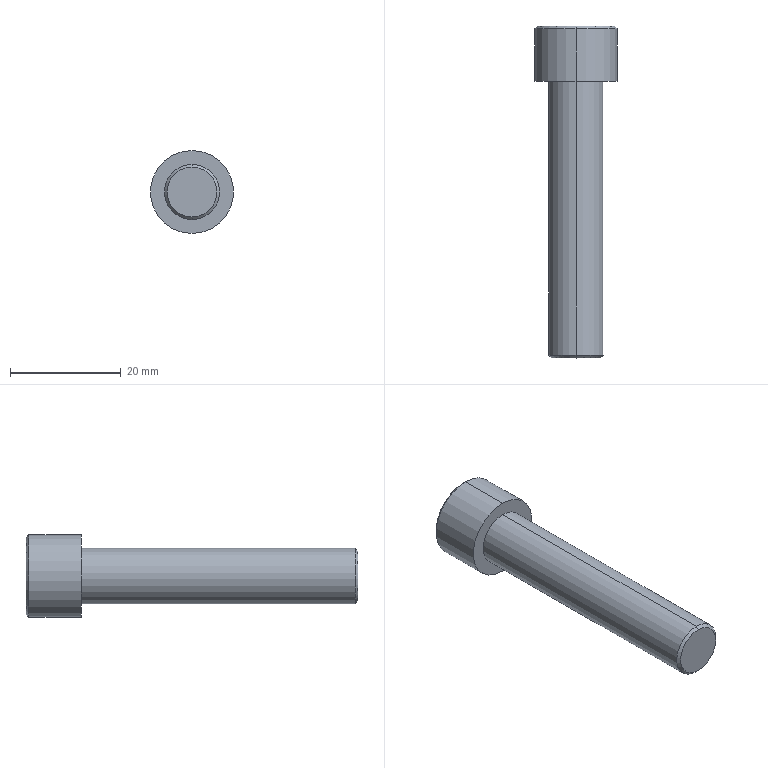Part | SolidWorks | features Chamfer 1, Extrusion 1, ICE 1 | 1 solid | 11 faces | box 15 x 60 x 15 mm | volume 5685 mm3 | cone 4 | cylinder 4 | plane 3 | commonest cylinder face diameters 10 x2 15 x2
STEP:
#1=CARTESIAN_POINT('',(0.,-25.,-4.5));
#2=VERTEX_POINT('',#1);
#3=CARTESIAN_POINT('',(0.,-25.,4.5));
#4=VERTEX_POINT('',#3);
#5=CARTESIAN_POINT('',(0.,-25.,0.));
#6=DIRECTION('',(0.,-1.,0.));
#7=DIRECTION('',(0.,0.,1.));
#8=AXIS2_PLACEMENT_3D('',#5,#6,#7);
#9=CIRCLE('',#8,4.5);
#10=EDGE_CURVE('',#2,#4,#9,.T.);
#11=ORIENTED_EDGE('',*,*,#10,.F.);
#12=CARTESIAN_POINT('',(0.,-24.5,-5.));
#13=VERTEX_POINT('',#12);
#14=CARTESIAN_POINT('',(0.,-24.5,-5.));
#15=DIRECTION('',(0.,0.7071,-0.7071));
#16=VECTOR('',#15,1000.);
#17=LINE('',#14,#16);
#18=EDGE_CURVE('',#2,#13,#17,.T.);
#19=ORIENTED_EDGE('',*,*,#18,.T.);
#20=CARTESIAN_POINT('',(0.,-24.5,5.));
#21=VERTEX_POINT('',#20);
#22=CARTESIAN_POINT('',(0.,-24.5,0.));
#23=DIRECTION('',(0.,1.,0.));
#24=DIRECTION('',(0.,0.,1.));
#25=AXIS2_PLACEMENT_3D('',#22,#23,#24);
#26=CIRCLE('',#25,5.);
#27=EDGE_CURVE('',#21,#13,#26,.T.);
#28=ORIENTED_EDGE('',*,*,#27,.F.);
#29=CARTESIAN_POINT('',(0.,-24.5,5.));
#30=DIRECTION('',(0.,0.7071,0.7071));
#31=VECTOR('',#30,1000.);
#32=LINE('',#29,#31);
#33=EDGE_CURVE('',#4,#21,#32,.T.);
#34=ORIENTED_EDGE('',*,*,#33,.F.);
#35=EDGE_LOOP('',(#11,#19,#28,#34));
#36=FACE_OUTER_BOUND('',#35,.T.);
#37=CARTESIAN_POINT('',(0.,-24.5,0.));
#38=DIRECTION('',(0.,1.,0.));
#39=DIRECTION('',(0.,0.,1.));
#40=AXIS2_PLACEMENT_3D('',#37,#38,#39);
#41=CONICAL_SURFACE('',#40,5.,0.7854);
#42=ADVANCED_FACE('',(#36),#41,.T.);
#43=CARTESIAN_POINT('',(0.,35.,7.));
#44=VERTEX_POINT('',#43);
#45=CARTESIAN_POINT('',(0.,35.,-7.));
#46=VERTEX_POINT('',#45);
#47=CARTESIAN_POINT('',(0.,35.,0.));
#48=DIRECTION('',(0.,1.,0.));
#49=DIRECTION('',(0.,0.,1.));
#50=AXIS2_PLACEMENT_3D('',#47,#48,#49);
#51=CIRCLE('',#50,7.);
#52=EDGE_CURVE('',#44,#46,#51,.T.);
#53=ORIENTED_EDGE('',*,*,#52,.F.);
#54=CARTESIAN_POINT('',(0.,34.5,7.5));
#55=VERTEX_POINT('',#54);
#56=CARTESIAN_POINT('',(0.,35.,7.));
#57=DIRECTION('',(0.,-0.7071,0.7071));
#58=VECTOR('',#57,1000.);
#59=LINE('',#56,#58);
#60=EDGE_CURVE('',#44,#55,#59,.T.);
#61=ORIENTED_EDGE('',*,*,#60,.T.);
#62=CARTESIAN_POINT('',(0.,34.5,-7.5));
#63=VERTEX_POINT('',#62);
#64=CARTESIAN_POINT('',(0.,34.5,0.));
#65=DIRECTION('',(0.,-1.,0.));
#66=DIRECTION('',(0.,0.,1.));
#67=AXIS2_PLACEMENT_3D('',#64,#65,#66);
#68=CIRCLE('',#67,7.5);
#69=EDGE_CURVE('',#63,#55,#68,.T.);
#70=ORIENTED_EDGE('',*,*,#69,.F.);
#71=CARTESIAN_POINT('',(0.,35.,-7.));
#72=DIRECTION('',(0.,-0.7071,-0.7071));
#73=VECTOR('',#72,1000.);
#74=LINE('',#71,#73);
#75=EDGE_CURVE('',#46,#63,#74,.T.);
#76=ORIENTED_EDGE('',*,*,#75,.F.);
#77=EDGE_LOOP('',(#53,#61,#70,#76));
#78=FACE_OUTER_BOUND('',#77,.T.);
#79=CARTESIAN_POINT('',(0.,35.,0.));
#80=DIRECTION('',(0.,-1.,0.));
#81=DIRECTION('',(0.,0.,-1.));
#82=AXIS2_PLACEMENT_3D('',#79,#80,#81);
#83=CONICAL_SURFACE('',#82,7.,0.7854);
#84=ADVANCED_FACE('',(#78),#83,.T.);
#85=ORIENTED_EDGE('',*,*,#69,.T.);
#86=CARTESIAN_POINT('',(0.,25.,7.5));
#87=VERTEX_POINT('',#86);
#88=CARTESIAN_POINT('',(0.,35.,7.5));
#89=DIRECTION('',(0.,-1.,0.));
#90=VECTOR('',#89,1000.);
#91=LINE('',#88,#90);
#92=EDGE_CURVE('',#55,#87,#91,.T.);
#93=ORIENTED_EDGE('',*,*,#92,.T.);
#94=CARTESIAN_POINT('',(0.,25.,-7.5));
#95=VERTEX_POINT('',#94);
#96=CARTESIAN_POINT('',(0.,25.,0.));
#97=DIRECTION('',(0.,1.,0.));
#98=DIRECTION('',(0.,0.,1.));
#99=AXIS2_PLACEMENT_3D('',#96,#97,#98);
#100=CIRCLE('',#99,7.5);
#101=EDGE_CURVE('',#87,#95,#100,.T.);
#102=ORIENTED_EDGE('',*,*,#101,.T.);
#103=CARTESIAN_POINT('',(0.,35.,-7.5));
#104=DIRECTION('',(0.,-1.,0.));
#105=VECTOR('',#104,1000.);
#106=LINE('',#103,#105);
#107=EDGE_CURVE('',#63,#95,#106,.T.);
#108=ORIENTED_EDGE('',*,*,#107,.F.);
#109=EDGE_LOOP('',(#85,#93,#102,#108));
#110=FACE_OUTER_BOUND('',#109,.T.);
#111=CARTESIAN_POINT('',(0.,35.,0.));
#112=DIRECTION('',(0.,-1.,0.));
#113=DIRECTION('',(0.,0.,-1.));
#114=AXIS2_PLACEMENT_3D('',#111,#112,#113);
#115=CYLINDRICAL_SURFACE('',#114,7.5);
#116=ADVANCED_FACE('',(#110),#115,.T.);
#117=CARTESIAN_POINT('',(0.,25.,5.));
#118=VERTEX_POINT('',#117);
#119=CARTESIAN_POINT('',(0.,25.,-5.));
#120=VERTEX_POINT('',#119);
#121=CARTESIAN_POINT('',(0.,25.,0.));
#122=DIRECTION('',(0.,1.,0.));
#123=DIRECTION('',(0.,0.,1.));
#124=AXIS2_PLACEMENT_3D('',#121,#122,#123);
#125=CIRCLE('',#124,5.);
#126=EDGE_CURVE('',#118,#120,#125,.T.);
#127=ORIENTED_EDGE('',*,*,#126,.F.);
#128=CARTESIAN_POINT('',(0.,25.,5.));
#129=DIRECTION('',(0.,-1.,0.));
#130=VECTOR('',#129,1000.);
#131=LINE('',#128,#130);
#132=EDGE_CURVE('',#118,#21,#131,.T.);
#133=ORIENTED_EDGE('',*,*,#132,.T.);
#134=ORIENTED_EDGE('',*,*,#27,.T.);
#135=CARTESIAN_POINT('',(0.,25.,-5.));
#136=DIRECTION('',(0.,-1.,0.));
#137=VECTOR('',#136,1000.);
#138=LINE('',#135,#137);
#139=EDGE_CURVE('',#120,#13,#138,.T.);
#140=ORIENTED_EDGE('',*,*,#139,.F.);
#141=EDGE_LOOP('',(#127,#133,#134,#140));
#142=FACE_OUTER_BOUND('',#141,.T.);
#143=CARTESIAN_POINT('',(0.,25.,0.));
#144=DIRECTION('',(0.,-1.,0.));
#145=DIRECTION('',(0.,0.,-1.));
#146=AXIS2_PLACEMENT_3D('',#143,#144,#145);
#147=CYLINDRICAL_SURFACE('',#146,5.);
#148=ADVANCED_FACE('',(#142),#147,.T.);
#149=ORIENTED_EDGE('',*,*,#132,.F.);
#150=CARTESIAN_POINT('',(0.,25.,0.));
#151=DIRECTION('',(0.,1.,0.));
#152=DIRECTION('',(0.,0.,1.));
#153=AXIS2_PLACEMENT_3D('',#150,#151,#152);
#154=CIRCLE('',#153,5.);
#155=EDGE_CURVE('',#120,#118,#154,.T.);
#156=ORIENTED_EDGE('',*,*,#155,.F.);
#157=ORIENTED_EDGE('',*,*,#139,.T.);
#158=CARTESIAN_POINT('',(0.,-24.5,0.));
#159=DIRECTION('',(0.,1.,0.));
#160=DIRECTION('',(0.,0.,1.));
#161=AXIS2_PLACEMENT_3D('',#158,#159,#160);
#162=CIRCLE('',#161,5.);
#163=EDGE_CURVE('',#13,#21,#162,.T.);
#164=ORIENTED_EDGE('',*,*,#163,.T.);
#165=EDGE_LOOP('',(#149,#156,#157,#164));
#166=FACE_OUTER_BOUND('',#165,.T.);
#167=CARTESIAN_POINT('',(0.,25.,0.));
#168=DIRECTION('',(0.,-1.,0.));
#169=DIRECTION('',(0.,0.,-1.));
#170=AXIS2_PLACEMENT_3D('',#167,#168,#169);
#171=CYLINDRICAL_SURFACE('',#170,5.);
#172=ADVANCED_FACE('',(#166),#171,.T.);
#173=CARTESIAN_POINT('',(0.,-25.,0.));
#174=DIRECTION('',(0.,-1.,0.));
#175=DIRECTION('',(0.,0.,1.));
#176=AXIS2_PLACEMENT_3D('',#173,#174,#175);
#177=CIRCLE('',#176,4.5);
#178=EDGE_CURVE('',#4,#2,#177,.T.);
#179=ORIENTED_EDGE('',*,*,#178,.T.);
#180=ORIENTED_EDGE('',*,*,#10,.T.);
#181=EDGE_LOOP('',(#179,#180));
#182=FACE_OUTER_BOUND('',#181,.T.);
#183=CARTESIAN_POINT('',(0.,-25.,0.));
#184=DIRECTION('',(0.,1.,0.));
#185=DIRECTION('',(0.,0.,1.));
#186=AXIS2_PLACEMENT_3D('',#183,#184,#185);
#187=PLANE('',#186);
#188=ADVANCED_FACE('',(#182),#187,.F.);
#189=ORIENTED_EDGE('',*,*,#92,.F.);
#190=CARTESIAN_POINT('',(0.,34.5,0.));
#191=DIRECTION('',(0.,-1.,0.));
#192=DIRECTION('',(0.,0.,1.));
#193=AXIS2_PLACEMENT_3D('',#190,#191,#192);
#194=CIRCLE('',#193,7.5);
#195=EDGE_CURVE('',#55,#63,#194,.T.);
#196=ORIENTED_EDGE('',*,*,#195,.T.);
#197=ORIENTED_EDGE('',*,*,#107,.T.);
#198=CARTESIAN_POINT('',(0.,25.,0.));
#199=DIRECTION('',(0.,1.,0.));
#200=DIRECTION('',(0.,0.,1.));
#201=AXIS2_PLACEMENT_3D('',#198,#199,#200);
#202=CIRCLE('',#201,7.5);
#203=EDGE_CURVE('',#95,#87,#202,.T.);
#204=ORIENTED_EDGE('',*,*,#203,.T.);
#205=EDGE_LOOP('',(#189,#196,#197,#204));
#206=FACE_OUTER_BOUND('',#205,.T.);
#207=CARTESIAN_POINT('',(0.,35.,0.));
#208=DIRECTION('',(0.,-1.,0.));
#209=DIRECTION('',(0.,0.,-1.));
#210=AXIS2_PLACEMENT_3D('',#207,#208,#209);
#211=CYLINDRICAL_SURFACE('',#210,7.5);
#212=ADVANCED_FACE('',(#206),#211,.T.);
#213=CARTESIAN_POINT('',(0.,35.,0.));
#214=DIRECTION('',(0.,1.,0.));
#215=DIRECTION('',(0.,0.,1.));
#216=AXIS2_PLACEMENT_3D('',#213,#214,#215);
#217=CIRCLE('',#216,7.);
#218=EDGE_CURVE('',#46,#44,#217,.T.);
#219=ORIENTED_EDGE('',*,*,#218,.T.);
#220=ORIENTED_EDGE('',*,*,#52,.T.);
#221=EDGE_LOOP('',(#219,#220));
#222=FACE_OUTER_BOUND('',#221,.T.);
#223=CARTESIAN_POINT('',(0.,35.,0.));
#224=DIRECTION('',(0.,1.,0.));
#225=DIRECTION('',(0.,0.,1.));
#226=AXIS2_PLACEMENT_3D('',#223,#224,#225);
#227=PLANE('',#226);
#228=ADVANCED_FACE('',(#222),#227,.T.);
#229=ORIENTED_EDGE('',*,*,#155,.T.);
#230=ORIENTED_EDGE('',*,*,#126,.T.);
#231=EDGE_LOOP('',(#229,#230));
#232=FACE_BOUND('',#231,.T.);
#233=ORIENTED_EDGE('',*,*,#203,.F.);
#234=ORIENTED_EDGE('',*,*,#101,.F.);
#235=EDGE_LOOP('',(#233,#234));
#236=FACE_OUTER_BOUND('',#235,.T.);
#237=CARTESIAN_POINT('',(0.,25.,0.));
#238=DIRECTION('',(0.,1.,0.));
#239=DIRECTION('',(0.,0.,1.));
#240=AXIS2_PLACEMENT_3D('',#237,#238,#239);
#241=PLANE('',#240);
#242=ADVANCED_FACE('',(#232,#236),#241,.F.);
#243=ORIENTED_EDGE('',*,*,#60,.F.);
#244=ORIENTED_EDGE('',*,*,#218,.F.);
#245=ORIENTED_EDGE('',*,*,#75,.T.);
#246=ORIENTED_EDGE('',*,*,#195,.F.);
#247=EDGE_LOOP('',(#243,#244,#245,#246));
#248=FACE_OUTER_BOUND('',#247,.T.);
#249=CARTESIAN_POINT('',(0.,35.,0.));
#250=DIRECTION('',(0.,-1.,0.));
#251=DIRECTION('',(0.,0.,-1.));
#252=AXIS2_PLACEMENT_3D('',#249,#250,#251);
#253=CONICAL_SURFACE('',#252,7.,0.7854);
#254=ADVANCED_FACE('',(#248),#253,.T.);
#255=ORIENTED_EDGE('',*,*,#18,.F.);
#256=ORIENTED_EDGE('',*,*,#178,.F.);
#257=ORIENTED_EDGE('',*,*,#33,.T.);
#258=ORIENTED_EDGE('',*,*,#163,.F.);
#259=EDGE_LOOP('',(#255,#256,#257,#258));
#260=FACE_OUTER_BOUND('',#259,.T.);
#261=CARTESIAN_POINT('',(0.,-24.5,0.));
#262=DIRECTION('',(0.,1.,0.));
#263=DIRECTION('',(0.,0.,1.));
#264=AXIS2_PLACEMENT_3D('',#261,#262,#263);
#265=CONICAL_SURFACE('',#264,5.,0.7854);
#266=ADVANCED_FACE('',(#260),#265,.T.);
#267=CLOSED_SHELL('',(#42,#84,#116,#148,#172,#188,#212,#228,#242,#254,#266));
#268=MANIFOLD_SOLID_BREP('',#267);
#269=CARTESIAN_POINT('',(0.,0.,0.));
#270=DIRECTION('',(0.,0.,1.));
#271=DIRECTION('',(1.,0.,0.));
#272=AXIS2_PLACEMENT_3D('',#269,#270,#271);
#273=(LENGTH_UNIT()NAMED_UNIT(*)SI_UNIT(.MILLI.,.METRE.));
#274=UNCERTAINTY_MEASURE_WITH_UNIT(LENGTH_MEASURE(0.00001),#273,'','');
#275=(NAMED_UNIT(*)PLANE_ANGLE_UNIT()SI_UNIT($,.RADIAN.));
#276=(NAMED_UNIT(*)SI_UNIT($,.STERADIAN.)SOLID_ANGLE_UNIT());
#277=(GEOMETRIC_REPRESENTATION_CONTEXT(3)GLOBAL_UNCERTAINTY_ASSIGNED_CONTEXT((#274))GLOBAL_UNIT_ASSIGNED_CONTEXT((#273,#275,#276))REPRESENTATION_CONTEXT('',''));
#278=ADVANCED_BREP_SHAPE_REPRESENTATION('',(#268,#272),#277);